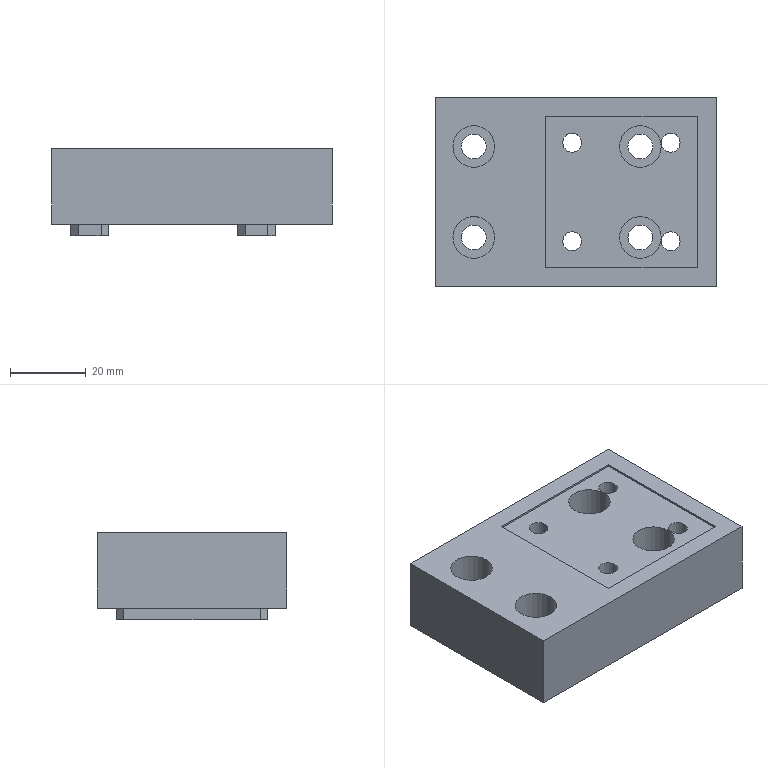Part | SolidWorks | features ICE 4, Chamfer 1, Extrusion 1 | 1 solid | 57 faces | box 74 x 50 x 23 mm | volume 67319 mm3 | plane 33 | cylinder 24 | commonest cylinder face diameters 5 x8 6.6 x8 11 x8